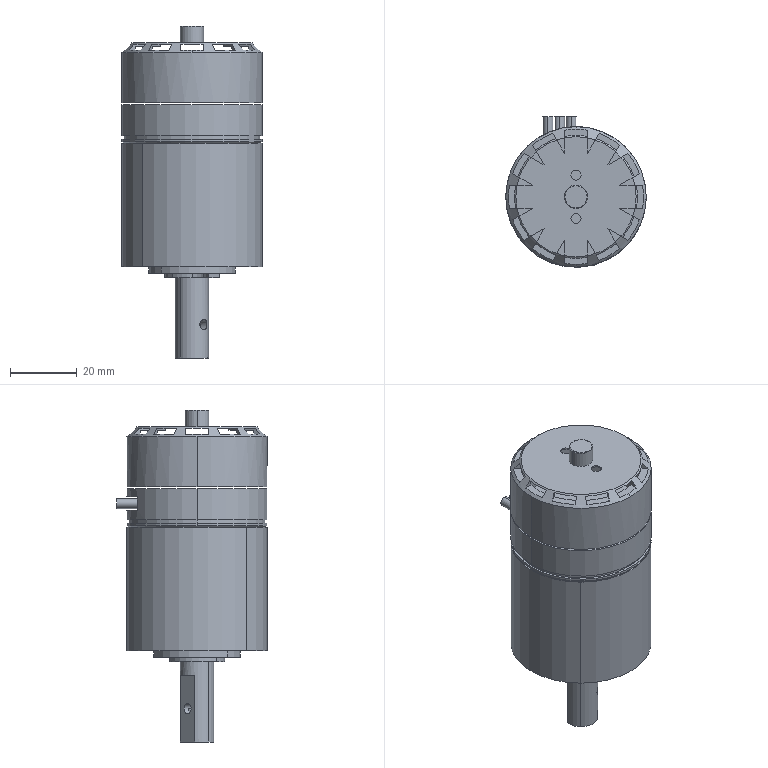Part | SolidWorks | 4 solids | 203 faces | box 42 x 45 x 99.3 mm | volume 75357 mm3 | plane 121 | cylinder 74 | cone 8 | commonest cylinder face diameters 3 x20 4 x16 5 x10 42 x8 10 x5 16.5 x3